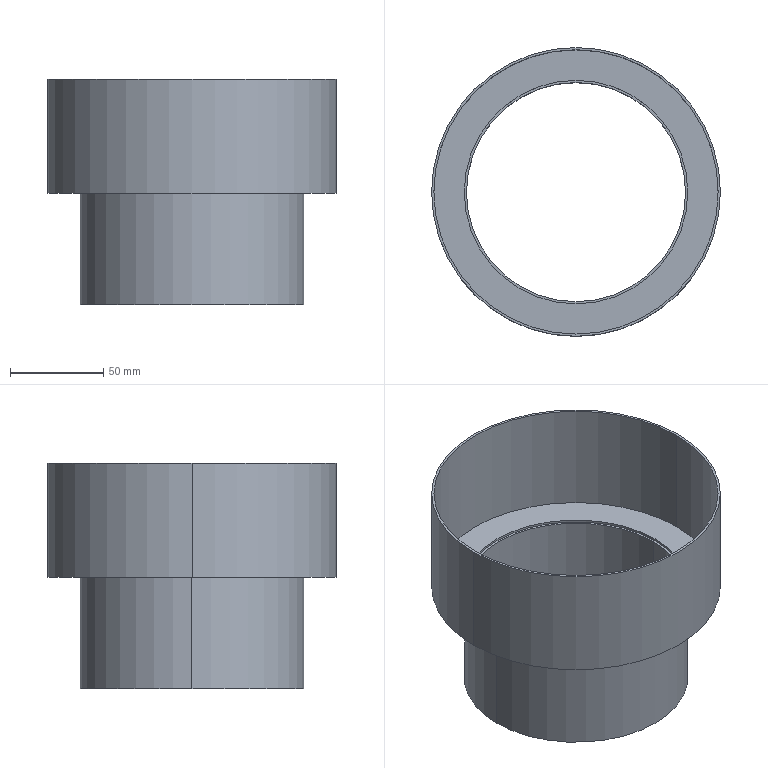Part | SolidWorks | features ICE 2, Extrusion 1 | 2 solids | 15 faces | box 155 x 155 x 121.2 mm | volume 70732 mm3 | cylinder 10 | plane 5 | commonest cylinder face diameters 120 x4 117.6 x2 152.6 x2 155 x2
STEP:
#1=CARTESIAN_POINT('',(60.,0.,-1.2));
#2=VERTEX_POINT('',#1);
#3=CARTESIAN_POINT('',(-60.,0.,-1.2));
#4=VERTEX_POINT('',#3);
#5=CARTESIAN_POINT('',(0.,0.,-1.2));
#6=DIRECTION('',(0.,0.,-1.));
#7=DIRECTION('',(-1.,0.,0.));
#8=AXIS2_PLACEMENT_3D('',#5,#6,#7);
#9=CIRCLE('',#8,60.);
#10=EDGE_CURVE('',#2,#4,#9,.T.);
#11=ORIENTED_EDGE('',*,*,#10,.T.);
#12=CARTESIAN_POINT('',(-60.,0.,0.));
#13=VERTEX_POINT('',#12);
#14=CARTESIAN_POINT('',(-60.,0.,-1.2));
#15=DIRECTION('',(0.,0.,1.));
#16=VECTOR('',#15,1000.);
#17=LINE('',#14,#16);
#18=EDGE_CURVE('',#4,#13,#17,.T.);
#19=ORIENTED_EDGE('',*,*,#18,.T.);
#20=CARTESIAN_POINT('',(60.,0.,0.));
#21=VERTEX_POINT('',#20);
#22=CARTESIAN_POINT('',(0.,0.,0.));
#23=DIRECTION('',(0.,0.,-1.));
#24=DIRECTION('',(-1.,0.,0.));
#25=AXIS2_PLACEMENT_3D('',#22,#23,#24);
#26=CIRCLE('',#25,60.);
#27=EDGE_CURVE('',#21,#13,#26,.T.);
#28=ORIENTED_EDGE('',*,*,#27,.F.);
#29=CARTESIAN_POINT('',(60.,0.,-1.2));
#30=DIRECTION('',(0.,0.,1.));
#31=VECTOR('',#30,1000.);
#32=LINE('',#29,#31);
#33=EDGE_CURVE('',#2,#21,#32,.T.);
#34=ORIENTED_EDGE('',*,*,#33,.F.);
#35=EDGE_LOOP('',(#11,#19,#28,#34));
#36=FACE_OUTER_BOUND('',#35,.T.);
#37=CARTESIAN_POINT('',(0.,0.,-1.2));
#38=DIRECTION('',(0.,0.,1.));
#39=DIRECTION('',(1.,0.,0.));
#40=AXIS2_PLACEMENT_3D('',#37,#38,#39);
#41=CYLINDRICAL_SURFACE('',#40,60.);
#42=ADVANCED_FACE('',(#36),#41,.F.);
#43=CARTESIAN_POINT('',(-76.3,0.,60.));
#44=VERTEX_POINT('',#43);
#45=CARTESIAN_POINT('',(76.3,0.,60.));
#46=VERTEX_POINT('',#45);
#47=CARTESIAN_POINT('',(0.,0.,60.));
#48=DIRECTION('',(0.,0.,1.));
#49=DIRECTION('',(1.,0.,0.));
#50=AXIS2_PLACEMENT_3D('',#47,#48,#49);
#51=CIRCLE('',#50,76.3);
#52=EDGE_CURVE('',#44,#46,#51,.T.);
#53=ORIENTED_EDGE('',*,*,#52,.T.);
#54=CARTESIAN_POINT('',(76.3,0.,0.));
#55=VERTEX_POINT('',#54);
#56=CARTESIAN_POINT('',(76.3,0.,60.));
#57=DIRECTION('',(0.,0.,-1.));
#58=VECTOR('',#57,1000.);
#59=LINE('',#56,#58);
#60=EDGE_CURVE('',#46,#55,#59,.T.);
#61=ORIENTED_EDGE('',*,*,#60,.T.);
#62=CARTESIAN_POINT('',(-76.3,0.,0.));
#63=VERTEX_POINT('',#62);
#64=CARTESIAN_POINT('',(0.,0.,0.));
#65=DIRECTION('',(0.,0.,1.));
#66=DIRECTION('',(1.,0.,0.));
#67=AXIS2_PLACEMENT_3D('',#64,#65,#66);
#68=CIRCLE('',#67,76.3);
#69=EDGE_CURVE('',#63,#55,#68,.T.);
#70=ORIENTED_EDGE('',*,*,#69,.F.);
#71=CARTESIAN_POINT('',(-76.3,0.,60.));
#72=DIRECTION('',(0.,0.,-1.));
#73=VECTOR('',#72,1000.);
#74=LINE('',#71,#73);
#75=EDGE_CURVE('',#44,#63,#74,.T.);
#76=ORIENTED_EDGE('',*,*,#75,.F.);
#77=EDGE_LOOP('',(#53,#61,#70,#76));
#78=FACE_OUTER_BOUND('',#77,.T.);
#79=CARTESIAN_POINT('',(0.,0.,60.));
#80=DIRECTION('',(0.,0.,-1.));
#81=DIRECTION('',(-1.,0.,0.));
#82=AXIS2_PLACEMENT_3D('',#79,#80,#81);
#83=CYLINDRICAL_SURFACE('',#82,76.3);
#84=ADVANCED_FACE('',(#78),#83,.F.);
#85=CARTESIAN_POINT('',(77.5,0.,60.));
#86=VERTEX_POINT('',#85);
#87=CARTESIAN_POINT('',(-77.5,0.,60.));
#88=VERTEX_POINT('',#87);
#89=CARTESIAN_POINT('',(0.,0.,60.));
#90=DIRECTION('',(0.,0.,1.));
#91=DIRECTION('',(1.,0.,0.));
#92=AXIS2_PLACEMENT_3D('',#89,#90,#91);
#93=CIRCLE('',#92,77.5);
#94=EDGE_CURVE('',#86,#88,#93,.T.);
#95=ORIENTED_EDGE('',*,*,#94,.F.);
#96=CARTESIAN_POINT('',(77.5,0.,-1.2));
#97=VERTEX_POINT('',#96);
#98=CARTESIAN_POINT('',(77.5,0.,60.));
#99=DIRECTION('',(0.,0.,-1.));
#100=VECTOR('',#99,1000.);
#101=LINE('',#98,#100);
#102=EDGE_CURVE('',#86,#97,#101,.T.);
#103=ORIENTED_EDGE('',*,*,#102,.T.);
#104=CARTESIAN_POINT('',(-77.5,0.,-1.2));
#105=VERTEX_POINT('',#104);
#106=CARTESIAN_POINT('',(0.,0.,-1.2));
#107=DIRECTION('',(0.,0.,-1.));
#108=DIRECTION('',(-1.,0.,0.));
#109=AXIS2_PLACEMENT_3D('',#106,#107,#108);
#110=CIRCLE('',#109,77.5);
#111=EDGE_CURVE('',#105,#97,#110,.T.);
#112=ORIENTED_EDGE('',*,*,#111,.F.);
#113=CARTESIAN_POINT('',(-77.5,0.,60.));
#114=DIRECTION('',(0.,0.,-1.));
#115=VECTOR('',#114,1000.);
#116=LINE('',#113,#115);
#117=EDGE_CURVE('',#88,#105,#116,.T.);
#118=ORIENTED_EDGE('',*,*,#117,.F.);
#119=EDGE_LOOP('',(#95,#103,#112,#118));
#120=FACE_OUTER_BOUND('',#119,.T.);
#121=CARTESIAN_POINT('',(0.,0.,60.));
#122=DIRECTION('',(0.,0.,-1.));
#123=DIRECTION('',(-1.,0.,0.));
#124=AXIS2_PLACEMENT_3D('',#121,#122,#123);
#125=CYLINDRICAL_SURFACE('',#124,77.5);
#126=ADVANCED_FACE('',(#120),#125,.T.);
#127=CARTESIAN_POINT('',(0.,0.,60.));
#128=DIRECTION('',(0.,0.,1.));
#129=DIRECTION('',(1.,0.,0.));
#130=AXIS2_PLACEMENT_3D('',#127,#128,#129);
#131=CIRCLE('',#130,77.5);
#132=EDGE_CURVE('',#88,#86,#131,.T.);
#133=ORIENTED_EDGE('',*,*,#132,.T.);
#134=ORIENTED_EDGE('',*,*,#94,.T.);
#135=EDGE_LOOP('',(#133,#134));
#136=FACE_OUTER_BOUND('',#135,.T.);
#137=ORIENTED_EDGE('',*,*,#52,.F.);
#138=CARTESIAN_POINT('',(0.,0.,60.));
#139=DIRECTION('',(0.,0.,1.));
#140=DIRECTION('',(1.,0.,0.));
#141=AXIS2_PLACEMENT_3D('',#138,#139,#140);
#142=CIRCLE('',#141,76.3);
#143=EDGE_CURVE('',#46,#44,#142,.T.);
#144=ORIENTED_EDGE('',*,*,#143,.F.);
#145=EDGE_LOOP('',(#137,#144));
#146=FACE_BOUND('',#145,.T.);
#147=CARTESIAN_POINT('',(0.,0.,60.));
#148=DIRECTION('',(0.,0.,1.));
#149=DIRECTION('',(1.,0.,0.));
#150=AXIS2_PLACEMENT_3D('',#147,#148,#149);
#151=PLANE('',#150);
#152=ADVANCED_FACE('',(#136,#146),#151,.T.);
#153=ORIENTED_EDGE('',*,*,#102,.F.);
#154=ORIENTED_EDGE('',*,*,#132,.F.);
#155=ORIENTED_EDGE('',*,*,#117,.T.);
#156=CARTESIAN_POINT('',(0.,0.,-1.2));
#157=DIRECTION('',(0.,0.,-1.));
#158=DIRECTION('',(-1.,0.,0.));
#159=AXIS2_PLACEMENT_3D('',#156,#157,#158);
#160=CIRCLE('',#159,77.5);
#161=EDGE_CURVE('',#97,#105,#160,.T.);
#162=ORIENTED_EDGE('',*,*,#161,.F.);
#163=EDGE_LOOP('',(#153,#154,#155,#162));
#164=FACE_OUTER_BOUND('',#163,.T.);
#165=CARTESIAN_POINT('',(0.,0.,60.));
#166=DIRECTION('',(0.,0.,-1.));
#167=DIRECTION('',(-1.,0.,0.));
#168=AXIS2_PLACEMENT_3D('',#165,#166,#167);
#169=CYLINDRICAL_SURFACE('',#168,77.5);
#170=ADVANCED_FACE('',(#164),#169,.T.);
#171=ORIENTED_EDGE('',*,*,#60,.F.);
#172=ORIENTED_EDGE('',*,*,#143,.T.);
#173=ORIENTED_EDGE('',*,*,#75,.T.);
#174=CARTESIAN_POINT('',(0.,0.,0.));
#175=DIRECTION('',(0.,0.,1.));
#176=DIRECTION('',(1.,0.,0.));
#177=AXIS2_PLACEMENT_3D('',#174,#175,#176);
#178=CIRCLE('',#177,76.3);
#179=EDGE_CURVE('',#55,#63,#178,.T.);
#180=ORIENTED_EDGE('',*,*,#179,.F.);
#181=EDGE_LOOP('',(#171,#172,#173,#180));
#182=FACE_OUTER_BOUND('',#181,.T.);
#183=CARTESIAN_POINT('',(0.,0.,60.));
#184=DIRECTION('',(0.,0.,-1.));
#185=DIRECTION('',(-1.,0.,0.));
#186=AXIS2_PLACEMENT_3D('',#183,#184,#185);
#187=CYLINDRICAL_SURFACE('',#186,76.3);
#188=ADVANCED_FACE('',(#182),#187,.F.);
#189=ORIENTED_EDGE('',*,*,#27,.T.);
#190=CARTESIAN_POINT('',(0.,0.,0.));
#191=DIRECTION('',(0.,0.,-1.));
#192=DIRECTION('',(-1.,0.,0.));
#193=AXIS2_PLACEMENT_3D('',#190,#191,#192);
#194=CIRCLE('',#193,60.);
#195=EDGE_CURVE('',#13,#21,#194,.T.);
#196=ORIENTED_EDGE('',*,*,#195,.T.);
#197=EDGE_LOOP('',(#189,#196));
#198=FACE_BOUND('',#197,.T.);
#199=ORIENTED_EDGE('',*,*,#69,.T.);
#200=ORIENTED_EDGE('',*,*,#179,.T.);
#201=EDGE_LOOP('',(#199,#200));
#202=FACE_OUTER_BOUND('',#201,.T.);
#203=CARTESIAN_POINT('',(0.,0.,0.));
#204=DIRECTION('',(0.,0.,-1.));
#205=DIRECTION('',(-1.,0.,0.));
#206=AXIS2_PLACEMENT_3D('',#203,#204,#205);
#207=PLANE('',#206);
#208=ADVANCED_FACE('',(#198,#202),#207,.F.);
#209=ORIENTED_EDGE('',*,*,#111,.T.);
#210=ORIENTED_EDGE('',*,*,#161,.T.);
#211=EDGE_LOOP('',(#209,#210));
#212=FACE_OUTER_BOUND('',#211,.T.);
#213=ORIENTED_EDGE('',*,*,#10,.F.);
#214=CARTESIAN_POINT('',(0.,0.,-1.2));
#215=DIRECTION('',(0.,0.,-1.));
#216=DIRECTION('',(-1.,0.,0.));
#217=AXIS2_PLACEMENT_3D('',#214,#215,#216);
#218=CIRCLE('',#217,60.);
#219=EDGE_CURVE('',#4,#2,#218,.T.);
#220=ORIENTED_EDGE('',*,*,#219,.F.);
#221=EDGE_LOOP('',(#213,#220));
#222=FACE_BOUND('',#221,.T.);
#223=CARTESIAN_POINT('',(0.,0.,-1.2));
#224=DIRECTION('',(0.,0.,-1.));
#225=DIRECTION('',(-1.,0.,0.));
#226=AXIS2_PLACEMENT_3D('',#223,#224,#225);
#227=PLANE('',#226);
#228=ADVANCED_FACE('',(#212,#222),#227,.T.);
#229=ORIENTED_EDGE('',*,*,#18,.F.);
#230=ORIENTED_EDGE('',*,*,#219,.T.);
#231=ORIENTED_EDGE('',*,*,#33,.T.);
#232=ORIENTED_EDGE('',*,*,#195,.F.);
#233=EDGE_LOOP('',(#229,#230,#231,#232));
#234=FACE_OUTER_BOUND('',#233,.T.);
#235=CARTESIAN_POINT('',(0.,0.,-1.2));
#236=DIRECTION('',(0.,0.,1.));
#237=DIRECTION('',(1.,0.,0.));
#238=AXIS2_PLACEMENT_3D('',#235,#236,#237);
#239=CYLINDRICAL_SURFACE('',#238,60.);
#240=ADVANCED_FACE('',(#234),#239,.F.);
#241=CLOSED_SHELL('',(#42,#84,#126,#152,#170,#188,#208,#228,#240));
#242=MANIFOLD_SOLID_BREP('',#241);
#243=CARTESIAN_POINT('',(58.8,0.,-61.2));
#244=VERTEX_POINT('',#243);
#245=CARTESIAN_POINT('',(-58.8,0.,-61.2));
#246=VERTEX_POINT('',#245);
#247=CARTESIAN_POINT('',(0.,0.,-61.2));
#248=DIRECTION('',(0.,0.,-1.));
#249=DIRECTION('',(-1.,0.,0.));
#250=AXIS2_PLACEMENT_3D('',#247,#248,#249);
#251=CIRCLE('',#250,58.8);
#252=EDGE_CURVE('',#244,#246,#251,.T.);
#253=ORIENTED_EDGE('',*,*,#252,.T.);
#254=CARTESIAN_POINT('',(-58.8,0.,-1.2));
#255=VERTEX_POINT('',#254);
#256=CARTESIAN_POINT('',(-58.8,0.,-61.2));
#257=DIRECTION('',(0.,0.,1.));
#258=VECTOR('',#257,1000.);
#259=LINE('',#256,#258);
#260=EDGE_CURVE('',#246,#255,#259,.T.);
#261=ORIENTED_EDGE('',*,*,#260,.T.);
#262=CARTESIAN_POINT('',(58.8,0.,-1.2));
#263=VERTEX_POINT('',#262);
#264=CARTESIAN_POINT('',(0.,0.,-1.2));
#265=DIRECTION('',(0.,0.,-1.));
#266=DIRECTION('',(-1.,0.,0.));
#267=AXIS2_PLACEMENT_3D('',#264,#265,#266);
#268=CIRCLE('',#267,58.8);
#269=EDGE_CURVE('',#263,#255,#268,.T.);
#270=ORIENTED_EDGE('',*,*,#269,.F.);
#271=CARTESIAN_POINT('',(58.8,0.,-61.2));
#272=DIRECTION('',(0.,0.,1.));
#273=VECTOR('',#272,1000.);
#274=LINE('',#271,#273);
#275=EDGE_CURVE('',#244,#263,#274,.T.);
#276=ORIENTED_EDGE('',*,*,#275,.F.);
#277=EDGE_LOOP('',(#253,#261,#270,#276));
#278=FACE_OUTER_BOUND('',#277,.T.);
#279=CARTESIAN_POINT('',(0.,0.,-61.2));
#280=DIRECTION('',(0.,0.,1.));
#281=DIRECTION('',(1.,0.,0.));
#282=AXIS2_PLACEMENT_3D('',#279,#280,#281);
#283=CYLINDRICAL_SURFACE('',#282,58.8);
#284=ADVANCED_FACE('',(#278),#283,.F.);
#285=CARTESIAN_POINT('',(-60.,0.,-61.2));
#286=VERTEX_POINT('',#285);
#287=CARTESIAN_POINT('',(60.,0.,-61.2));
#288=VERTEX_POINT('',#287);
#289=CARTESIAN_POINT('',(0.,0.,-61.2));
#290=DIRECTION('',(0.,0.,-1.));
#291=DIRECTION('',(-1.,0.,0.));
#292=AXIS2_PLACEMENT_3D('',#289,#290,#291);
#293=CIRCLE('',#292,60.);
#294=EDGE_CURVE('',#286,#288,#293,.T.);
#295=ORIENTED_EDGE('',*,*,#294,.F.);
#296=CARTESIAN_POINT('',(-60.,0.,-1.2));
#297=VERTEX_POINT('',#296);
#298=CARTESIAN_POINT('',(-60.,0.,-61.2));
#299=DIRECTION('',(0.,0.,1.));
#300=VECTOR('',#299,1000.);
#301=LINE('',#298,#300);
#302=EDGE_CURVE('',#286,#297,#301,.T.);
#303=ORIENTED_EDGE('',*,*,#302,.T.);
#304=CARTESIAN_POINT('',(60.,0.,-1.2));
#305=VERTEX_POINT('',#304);
#306=CARTESIAN_POINT('',(0.,0.,-1.2));
#307=DIRECTION('',(0.,0.,-1.));
#308=DIRECTION('',(-1.,0.,0.));
#309=AXIS2_PLACEMENT_3D('',#306,#307,#308);
#310=CIRCLE('',#309,60.);
#311=EDGE_CURVE('',#297,#305,#310,.T.);
#312=ORIENTED_EDGE('',*,*,#311,.T.);
#313=CARTESIAN_POINT('',(60.,0.,-61.2));
#314=DIRECTION('',(0.,0.,1.));
#315=VECTOR('',#314,1000.);
#316=LINE('',#313,#315);
#317=EDGE_CURVE('',#288,#305,#316,.T.);
#318=ORIENTED_EDGE('',*,*,#317,.F.);
#319=EDGE_LOOP('',(#295,#303,#312,#318));
#320=FACE_OUTER_BOUND('',#319,.T.);
#321=CARTESIAN_POINT('',(0.,0.,-61.2));
#322=DIRECTION('',(0.,0.,1.));
#323=DIRECTION('',(1.,0.,0.));
#324=AXIS2_PLACEMENT_3D('',#321,#322,#323);
#325=CYLINDRICAL_SURFACE('',#324,60.);
#326=ADVANCED_FACE('',(#320),#325,.T.);
#327=CARTESIAN_POINT('',(0.,0.,-61.2));
#328=DIRECTION('',(0.,0.,-1.));
#329=DIRECTION('',(-1.,0.,0.));
#330=AXIS2_PLACEMENT_3D('',#327,#328,#329);
#331=CIRCLE('',#330,60.);
#332=EDGE_CURVE('',#288,#286,#331,.T.);
#333=ORIENTED_EDGE('',*,*,#332,.T.);
#334=ORIENTED_EDGE('',*,*,#294,.T.);
#335=EDGE_LOOP('',(#333,#334));
#336=FACE_OUTER_BOUND('',#335,.T.);
#337=ORIENTED_EDGE('',*,*,#252,.F.);
#338=CARTESIAN_POINT('',(0.,0.,-61.2));
#339=DIRECTION('',(0.,0.,-1.));
#340=DIRECTION('',(-1.,0.,0.));
#341=AXIS2_PLACEMENT_3D('',#338,#339,#340);
#342=CIRCLE('',#341,58.8);
#343=EDGE_CURVE('',#246,#244,#342,.T.);
#344=ORIENTED_EDGE('',*,*,#343,.F.);
#345=EDGE_LOOP('',(#337,#344));
#346=FACE_BOUND('',#345,.T.);
#347=CARTESIAN_POINT('',(0.,0.,-61.2));
#348=DIRECTION('',(0.,0.,-1.));
#349=DIRECTION('',(-1.,0.,0.));
#350=AXIS2_PLACEMENT_3D('',#347,#348,#349);
#351=PLANE('',#350);
#352=ADVANCED_FACE('',(#336,#346),#351,.T.);
#353=CARTESIAN_POINT('',(0.,0.,-1.2));
#354=DIRECTION('',(0.,0.,-1.));
#355=DIRECTION('',(-1.,0.,0.));
#356=AXIS2_PLACEMENT_3D('',#353,#354,#355);
#357=CIRCLE('',#356,60.);
#358=EDGE_CURVE('',#305,#297,#357,.T.);
#359=ORIENTED_EDGE('',*,*,#358,.F.);
#360=ORIENTED_EDGE('',*,*,#311,.F.);
#361=EDGE_LOOP('',(#359,#360));
#362=FACE_OUTER_BOUND('',#361,.T.);
#363=ORIENTED_EDGE('',*,*,#269,.T.);
#364=CARTESIAN_POINT('',(0.,0.,-1.2));
#365=DIRECTION('',(0.,0.,-1.));
#366=DIRECTION('',(-1.,0.,0.));
#367=AXIS2_PLACEMENT_3D('',#364,#365,#366);
#368=CIRCLE('',#367,58.8);
#369=EDGE_CURVE('',#255,#263,#368,.T.);
#370=ORIENTED_EDGE('',*,*,#369,.T.);
#371=EDGE_LOOP('',(#363,#370));
#372=FACE_BOUND('',#371,.T.);
#373=CARTESIAN_POINT('',(0.,0.,-1.2));
#374=DIRECTION('',(0.,0.,-1.));
#375=DIRECTION('',(-1.,0.,0.));
#376=AXIS2_PLACEMENT_3D('',#373,#374,#375);
#377=PLANE('',#376);
#378=ADVANCED_FACE('',(#362,#372),#377,.F.);
#379=ORIENTED_EDGE('',*,*,#302,.F.);
#380=ORIENTED_EDGE('',*,*,#332,.F.);
#381=ORIENTED_EDGE('',*,*,#317,.T.);
#382=ORIENTED_EDGE('',*,*,#358,.T.);
#383=EDGE_LOOP('',(#379,#380,#381,#382));
#384=FACE_OUTER_BOUND('',#383,.T.);
#385=CARTESIAN_POINT('',(0.,0.,-61.2));
#386=DIRECTION('',(0.,0.,1.));
#387=DIRECTION('',(1.,0.,0.));
#388=AXIS2_PLACEMENT_3D('',#385,#386,#387);
#389=CYLINDRICAL_SURFACE('',#388,60.);
#390=ADVANCED_FACE('',(#384),#389,.T.);
#391=ORIENTED_EDGE('',*,*,#260,.F.);
#392=ORIENTED_EDGE('',*,*,#343,.T.);
#393=ORIENTED_EDGE('',*,*,#275,.T.);
#394=ORIENTED_EDGE('',*,*,#369,.F.);
#395=EDGE_LOOP('',(#391,#392,#393,#394));
#396=FACE_OUTER_BOUND('',#395,.T.);
#397=CARTESIAN_POINT('',(0.,0.,-61.2));
#398=DIRECTION('',(0.,0.,1.));
#399=DIRECTION('',(1.,0.,0.));
#400=AXIS2_PLACEMENT_3D('',#397,#398,#399);
#401=CYLINDRICAL_SURFACE('',#400,58.8);
#402=ADVANCED_FACE('',(#396),#401,.F.);
#403=CLOSED_SHELL('',(#284,#326,#352,#378,#390,#402));
#404=MANIFOLD_SOLID_BREP('',#403);
#405=CARTESIAN_POINT('',(0.,0.,0.));
#406=DIRECTION('',(0.,0.,1.));
#407=DIRECTION('',(1.,0.,0.));
#408=AXIS2_PLACEMENT_3D('',#405,#406,#407);
#409=(LENGTH_UNIT()NAMED_UNIT(*)SI_UNIT(.MILLI.,.METRE.));
#410=UNCERTAINTY_MEASURE_WITH_UNIT(LENGTH_MEASURE(0.00001),#409,'','');
#411=(NAMED_UNIT(*)PLANE_ANGLE_UNIT()SI_UNIT($,.RADIAN.));
#412=(NAMED_UNIT(*)SI_UNIT($,.STERADIAN.)SOLID_ANGLE_UNIT());
#413=(GEOMETRIC_REPRESENTATION_CONTEXT(3)GLOBAL_UNCERTAINTY_ASSIGNED_CONTEXT((#410))GLOBAL_UNIT_ASSIGNED_CONTEXT((#409,#411,#412))REPRESENTATION_CONTEXT('',''));
#414=ADVANCED_BREP_SHAPE_REPRESENTATION('',(#242,#404,#408),#413);